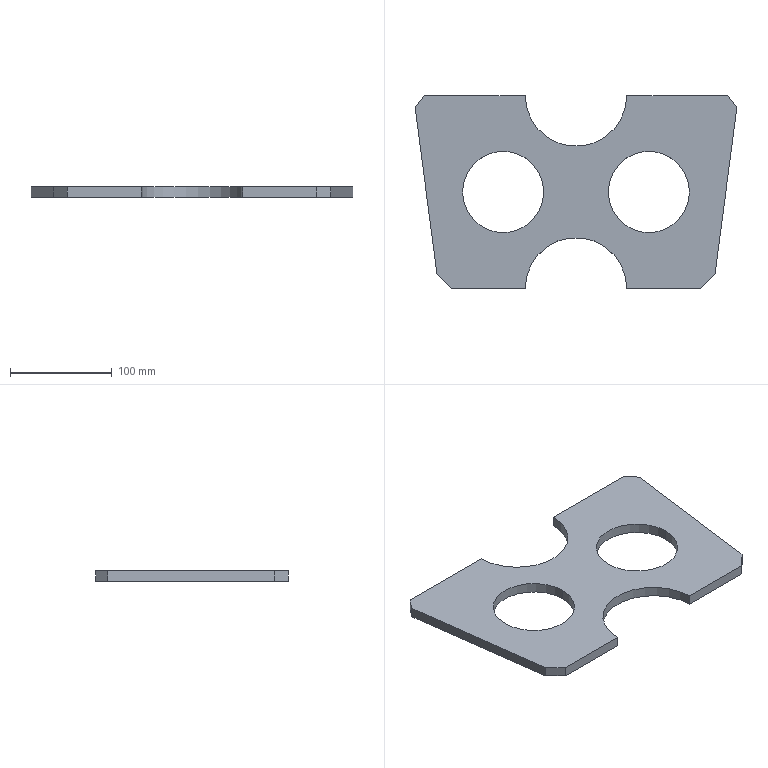Part | SolidWorks | features Extrusion 1 | 1 solid | 18 faces | box 316.869 x 190 x 10 mm | volume 378498 mm3 | plane 12 | cylinder 6 | commonest cylinder face diameters 80 x4 100 x2
STEP:
#1=CARTESIAN_POINT('',(-31.75,0.,10.));
#2=VERTEX_POINT('',#1);
#3=CARTESIAN_POINT('',(-111.75,0.,10.));
#4=VERTEX_POINT('',#3);
#5=CARTESIAN_POINT('',(-71.75,0.,10.));
#6=DIRECTION('',(0.,0.,-1.));
#7=DIRECTION('',(1.,0.,0.));
#8=AXIS2_PLACEMENT_3D('',#5,#6,#7);
#9=CIRCLE('',#8,40.);
#10=EDGE_CURVE('',#2,#4,#9,.T.);
#11=ORIENTED_EDGE('',*,*,#10,.F.);
#12=CARTESIAN_POINT('',(-31.75,0.,0.));
#13=VERTEX_POINT('',#12);
#14=CARTESIAN_POINT('',(-31.75,0.,10.));
#15=DIRECTION('',(0.,0.,-1.));
#16=VECTOR('',#15,1000.);
#17=LINE('',#14,#16);
#18=EDGE_CURVE('',#2,#13,#17,.T.);
#19=ORIENTED_EDGE('',*,*,#18,.T.);
#20=CARTESIAN_POINT('',(-111.75,0.,0.));
#21=VERTEX_POINT('',#20);
#22=CARTESIAN_POINT('',(-71.75,0.,0.));
#23=DIRECTION('',(0.,0.,-1.));
#24=DIRECTION('',(1.,0.,0.));
#25=AXIS2_PLACEMENT_3D('',#22,#23,#24);
#26=CIRCLE('',#25,40.);
#27=EDGE_CURVE('',#13,#21,#26,.T.);
#28=ORIENTED_EDGE('',*,*,#27,.T.);
#29=CARTESIAN_POINT('',(-111.75,0.,10.));
#30=DIRECTION('',(0.,0.,-1.));
#31=VECTOR('',#30,1000.);
#32=LINE('',#29,#31);
#33=EDGE_CURVE('',#4,#21,#32,.T.);
#34=ORIENTED_EDGE('',*,*,#33,.F.);
#35=EDGE_LOOP('',(#11,#19,#28,#34));
#36=FACE_OUTER_BOUND('',#35,.T.);
#37=CARTESIAN_POINT('',(-71.75,0.,10.));
#38=DIRECTION('',(0.,0.,-1.));
#39=DIRECTION('',(-1.,0.,0.));
#40=AXIS2_PLACEMENT_3D('',#37,#38,#39);
#41=CYLINDRICAL_SURFACE('',#40,40.);
#42=ADVANCED_FACE('',(#36),#41,.F.);
#43=CARTESIAN_POINT('',(31.75,0.,10.));
#44=VERTEX_POINT('',#43);
#45=CARTESIAN_POINT('',(111.75,0.,10.));
#46=VERTEX_POINT('',#45);
#47=CARTESIAN_POINT('',(71.75,0.,10.));
#48=DIRECTION('',(0.,0.,1.));
#49=DIRECTION('',(1.,0.,0.));
#50=AXIS2_PLACEMENT_3D('',#47,#48,#49);
#51=CIRCLE('',#50,40.);
#52=EDGE_CURVE('',#44,#46,#51,.T.);
#53=ORIENTED_EDGE('',*,*,#52,.T.);
#54=CARTESIAN_POINT('',(111.75,0.,0.));
#55=VERTEX_POINT('',#54);
#56=CARTESIAN_POINT('',(111.75,0.,10.));
#57=DIRECTION('',(0.,0.,-1.));
#58=VECTOR('',#57,1000.);
#59=LINE('',#56,#58);
#60=EDGE_CURVE('',#46,#55,#59,.T.);
#61=ORIENTED_EDGE('',*,*,#60,.T.);
#62=CARTESIAN_POINT('',(31.75,0.,0.));
#63=VERTEX_POINT('',#62);
#64=CARTESIAN_POINT('',(71.75,0.,0.));
#65=DIRECTION('',(0.,0.,1.));
#66=DIRECTION('',(1.,0.,0.));
#67=AXIS2_PLACEMENT_3D('',#64,#65,#66);
#68=CIRCLE('',#67,40.);
#69=EDGE_CURVE('',#63,#55,#68,.T.);
#70=ORIENTED_EDGE('',*,*,#69,.F.);
#71=CARTESIAN_POINT('',(31.75,0.,10.));
#72=DIRECTION('',(0.,0.,-1.));
#73=VECTOR('',#72,1000.);
#74=LINE('',#71,#73);
#75=EDGE_CURVE('',#44,#63,#74,.T.);
#76=ORIENTED_EDGE('',*,*,#75,.F.);
#77=EDGE_LOOP('',(#53,#61,#70,#76));
#78=FACE_OUTER_BOUND('',#77,.T.);
#79=CARTESIAN_POINT('',(71.75,0.,10.));
#80=DIRECTION('',(0.,0.,-1.));
#81=DIRECTION('',(-1.,0.,0.));
#82=AXIS2_PLACEMENT_3D('',#79,#80,#81);
#83=CYLINDRICAL_SURFACE('',#82,40.);
#84=ADVANCED_FACE('',(#78),#83,.F.);
#85=CARTESIAN_POINT('',(50.,-95.,0.));
#86=VERTEX_POINT('',#85);
#87=CARTESIAN_POINT('',(-50.,-95.,0.));
#88=VERTEX_POINT('',#87);
#89=CARTESIAN_POINT('',(0.,-95.,0.));
#90=DIRECTION('',(0.,0.,1.));
#91=DIRECTION('',(1.,0.,0.));
#92=AXIS2_PLACEMENT_3D('',#89,#90,#91);
#93=CIRCLE('',#92,50.);
#94=EDGE_CURVE('',#86,#88,#93,.T.);
#95=ORIENTED_EDGE('',*,*,#94,.F.);
#96=CARTESIAN_POINT('',(50.,-95.,10.));
#97=VERTEX_POINT('',#96);
#98=CARTESIAN_POINT('',(50.,-95.,10.));
#99=DIRECTION('',(0.,0.,-1.));
#100=VECTOR('',#99,1000.);
#101=LINE('',#98,#100);
#102=EDGE_CURVE('',#97,#86,#101,.T.);
#103=ORIENTED_EDGE('',*,*,#102,.F.);
#104=CARTESIAN_POINT('',(-50.,-95.,10.));
#105=VERTEX_POINT('',#104);
#106=CARTESIAN_POINT('',(0.,-95.,10.));
#107=DIRECTION('',(0.,0.,1.));
#108=DIRECTION('',(1.,0.,0.));
#109=AXIS2_PLACEMENT_3D('',#106,#107,#108);
#110=CIRCLE('',#109,50.);
#111=EDGE_CURVE('',#97,#105,#110,.T.);
#112=ORIENTED_EDGE('',*,*,#111,.T.);
#113=CARTESIAN_POINT('',(-50.,-95.,10.));
#114=DIRECTION('',(0.,0.,-1.));
#115=VECTOR('',#114,1000.);
#116=LINE('',#113,#115);
#117=EDGE_CURVE('',#105,#88,#116,.T.);
#118=ORIENTED_EDGE('',*,*,#117,.T.);
#119=EDGE_LOOP('',(#95,#103,#112,#118));
#120=FACE_OUTER_BOUND('',#119,.T.);
#121=CARTESIAN_POINT('',(0.,-95.,10.));
#122=DIRECTION('',(0.,0.,-1.));
#123=DIRECTION('',(-1.,0.,0.));
#124=AXIS2_PLACEMENT_3D('',#121,#122,#123);
#125=CYLINDRICAL_SURFACE('',#124,50.);
#126=ADVANCED_FACE('',(#120),#125,.F.);
#127=CARTESIAN_POINT('',(123.,-95.,0.));
#128=VERTEX_POINT('',#127);
#129=CARTESIAN_POINT('',(0.,-95.,0.));
#130=DIRECTION('',(1.,0.,0.));
#131=VECTOR('',#130,1000.);
#132=LINE('',#129,#131);
#133=EDGE_CURVE('',#86,#128,#132,.T.);
#134=ORIENTED_EDGE('',*,*,#133,.T.);
#135=CARTESIAN_POINT('',(123.,-95.,10.));
#136=VERTEX_POINT('',#135);
#137=CARTESIAN_POINT('',(123.,-95.,10.));
#138=DIRECTION('',(0.,0.,-1.));
#139=VECTOR('',#138,1000.);
#140=LINE('',#137,#139);
#141=EDGE_CURVE('',#136,#128,#140,.T.);
#142=ORIENTED_EDGE('',*,*,#141,.F.);
#143=CARTESIAN_POINT('',(0.,-95.,10.));
#144=DIRECTION('',(1.,0.,0.));
#145=VECTOR('',#144,1000.);
#146=LINE('',#143,#145);
#147=EDGE_CURVE('',#97,#136,#146,.T.);
#148=ORIENTED_EDGE('',*,*,#147,.F.);
#149=ORIENTED_EDGE('',*,*,#102,.T.);
#150=EDGE_LOOP('',(#134,#142,#148,#149));
#151=FACE_OUTER_BOUND('',#150,.T.);
#152=CARTESIAN_POINT('',(0.,-95.,10.));
#153=DIRECTION('',(0.,1.,0.));
#154=DIRECTION('',(0.,0.,1.));
#155=AXIS2_PLACEMENT_3D('',#152,#153,#154);
#156=PLANE('',#155);
#157=ADVANCED_FACE('',(#151),#156,.F.);
#158=CARTESIAN_POINT('',(136.818,-81.182,0.));
#159=VERTEX_POINT('',#158);
#160=CARTESIAN_POINT('',(-34.76,-252.76,0.));
#161=DIRECTION('',(0.7071,0.7071,0.));
#162=VECTOR('',#161,1000.);
#163=LINE('',#160,#162);
#164=EDGE_CURVE('',#128,#159,#163,.T.);
#165=ORIENTED_EDGE('',*,*,#164,.T.);
#166=CARTESIAN_POINT('',(136.818,-81.182,10.));
#167=VERTEX_POINT('',#166);
#168=CARTESIAN_POINT('',(136.818,-81.182,10.));
#169=DIRECTION('',(0.,0.,-1.));
#170=VECTOR('',#169,1000.);
#171=LINE('',#168,#170);
#172=EDGE_CURVE('',#167,#159,#171,.T.);
#173=ORIENTED_EDGE('',*,*,#172,.F.);
#174=CARTESIAN_POINT('',(-34.76,-252.76,10.));
#175=DIRECTION('',(0.7071,0.7071,0.));
#176=VECTOR('',#175,1000.);
#177=LINE('',#174,#176);
#178=EDGE_CURVE('',#136,#167,#177,.T.);
#179=ORIENTED_EDGE('',*,*,#178,.F.);
#180=ORIENTED_EDGE('',*,*,#141,.T.);
#181=EDGE_LOOP('',(#165,#173,#179,#180));
#182=FACE_OUTER_BOUND('',#181,.T.);
#183=CARTESIAN_POINT('',(-34.76,-252.76,10.));
#184=DIRECTION('',(-0.7071,0.7071,0.));
#185=DIRECTION('',(-0.7071,-0.7071,0.));
#186=AXIS2_PLACEMENT_3D('',#183,#184,#185);
#187=PLANE('',#186);
#188=ADVANCED_FACE('',(#182),#187,.F.);
#189=CARTESIAN_POINT('',(158.435,83.103,0.));
#190=VERTEX_POINT('',#189);
#191=CARTESIAN_POINT('',(107.802,-301.704,0.));
#192=DIRECTION('',(-0.1305,-0.9915,0.));
#193=VECTOR('',#192,1000.);
#194=LINE('',#191,#193);
#195=EDGE_CURVE('',#190,#159,#194,.T.);
#196=ORIENTED_EDGE('',*,*,#195,.F.);
#197=CARTESIAN_POINT('',(158.435,83.103,10.));
#198=VERTEX_POINT('',#197);
#199=CARTESIAN_POINT('',(158.435,83.103,10.));
#200=DIRECTION('',(0.,0.,-1.));
#201=VECTOR('',#200,1000.);
#202=LINE('',#199,#201);
#203=EDGE_CURVE('',#198,#190,#202,.T.);
#204=ORIENTED_EDGE('',*,*,#203,.F.);
#205=CARTESIAN_POINT('',(107.802,-301.704,10.));
#206=DIRECTION('',(-0.1305,-0.9915,0.));
#207=VECTOR('',#206,1000.);
#208=LINE('',#205,#207);
#209=EDGE_CURVE('',#198,#167,#208,.T.);
#210=ORIENTED_EDGE('',*,*,#209,.T.);
#211=ORIENTED_EDGE('',*,*,#172,.T.);
#212=EDGE_LOOP('',(#196,#204,#210,#211));
#213=FACE_OUTER_BOUND('',#212,.T.);
#214=CARTESIAN_POINT('',(107.802,-301.704,10.));
#215=DIRECTION('',(0.9915,-0.1305,0.));
#216=DIRECTION('',(0.1305,0.9915,0.));
#217=AXIS2_PLACEMENT_3D('',#214,#215,#216);
#218=PLANE('',#217);
#219=ADVANCED_FACE('',(#213),#218,.T.);
#220=CARTESIAN_POINT('',(149.304,95.,0.));
#221=VERTEX_POINT('',#220);
#222=CARTESIAN_POINT('',(278.713,-73.624,0.));
#223=DIRECTION('',(0.6088,-0.7933,0.));
#224=VECTOR('',#223,1000.);
#225=LINE('',#222,#224);
#226=EDGE_CURVE('',#221,#190,#225,.T.);
#227=ORIENTED_EDGE('',*,*,#226,.F.);
#228=CARTESIAN_POINT('',(149.304,95.,10.));
#229=VERTEX_POINT('',#228);
#230=CARTESIAN_POINT('',(149.304,95.,10.));
#231=DIRECTION('',(0.,0.,-1.));
#232=VECTOR('',#231,1000.);
#233=LINE('',#230,#232);
#234=EDGE_CURVE('',#229,#221,#233,.T.);
#235=ORIENTED_EDGE('',*,*,#234,.F.);
#236=CARTESIAN_POINT('',(278.713,-73.624,10.));
#237=DIRECTION('',(0.6088,-0.7933,0.));
#238=VECTOR('',#237,1000.);
#239=LINE('',#236,#238);
#240=EDGE_CURVE('',#229,#198,#239,.T.);
#241=ORIENTED_EDGE('',*,*,#240,.T.);
#242=ORIENTED_EDGE('',*,*,#203,.T.);
#243=EDGE_LOOP('',(#227,#235,#241,#242));
#244=FACE_OUTER_BOUND('',#243,.T.);
#245=CARTESIAN_POINT('',(278.713,-73.624,10.));
#246=DIRECTION('',(0.7933,0.6088,0.));
#247=DIRECTION('',(-0.6088,0.7933,0.));
#248=AXIS2_PLACEMENT_3D('',#245,#246,#247);
#249=PLANE('',#248);
#250=ADVANCED_FACE('',(#244),#249,.T.);
#251=CARTESIAN_POINT('',(50.,95.,0.));
#252=VERTEX_POINT('',#251);
#253=CARTESIAN_POINT('',(0.,95.,0.));
#254=DIRECTION('',(1.,0.,0.));
#255=VECTOR('',#254,1000.);
#256=LINE('',#253,#255);
#257=EDGE_CURVE('',#252,#221,#256,.T.);
#258=ORIENTED_EDGE('',*,*,#257,.F.);
#259=CARTESIAN_POINT('',(50.,95.,10.));
#260=VERTEX_POINT('',#259);
#261=CARTESIAN_POINT('',(50.,95.,10.));
#262=DIRECTION('',(0.,0.,-1.));
#263=VECTOR('',#262,1000.);
#264=LINE('',#261,#263);
#265=EDGE_CURVE('',#260,#252,#264,.T.);
#266=ORIENTED_EDGE('',*,*,#265,.F.);
#267=CARTESIAN_POINT('',(0.,95.,10.));
#268=DIRECTION('',(1.,0.,0.));
#269=VECTOR('',#268,1000.);
#270=LINE('',#267,#269);
#271=EDGE_CURVE('',#260,#229,#270,.T.);
#272=ORIENTED_EDGE('',*,*,#271,.T.);
#273=ORIENTED_EDGE('',*,*,#234,.T.);
#274=EDGE_LOOP('',(#258,#266,#272,#273));
#275=FACE_OUTER_BOUND('',#274,.T.);
#276=CARTESIAN_POINT('',(0.,95.,10.));
#277=DIRECTION('',(0.,1.,0.));
#278=DIRECTION('',(0.,0.,1.));
#279=AXIS2_PLACEMENT_3D('',#276,#277,#278);
#280=PLANE('',#279);
#281=ADVANCED_FACE('',(#275),#280,.T.);
#282=CARTESIAN_POINT('',(-50.,95.,0.));
#283=VERTEX_POINT('',#282);
#284=CARTESIAN_POINT('',(0.,95.,0.));
#285=DIRECTION('',(0.,0.,1.));
#286=DIRECTION('',(1.,0.,0.));
#287=AXIS2_PLACEMENT_3D('',#284,#285,#286);
#288=CIRCLE('',#287,50.);
#289=EDGE_CURVE('',#283,#252,#288,.T.);
#290=ORIENTED_EDGE('',*,*,#289,.F.);
#291=CARTESIAN_POINT('',(-50.,95.,10.));
#292=VERTEX_POINT('',#291);
#293=CARTESIAN_POINT('',(-50.,95.,10.));
#294=DIRECTION('',(0.,0.,-1.));
#295=VECTOR('',#294,1000.);
#296=LINE('',#293,#295);
#297=EDGE_CURVE('',#292,#283,#296,.T.);
#298=ORIENTED_EDGE('',*,*,#297,.F.);
#299=CARTESIAN_POINT('',(0.,95.,10.));
#300=DIRECTION('',(0.,0.,1.));
#301=DIRECTION('',(1.,0.,0.));
#302=AXIS2_PLACEMENT_3D('',#299,#300,#301);
#303=CIRCLE('',#302,50.);
#304=EDGE_CURVE('',#292,#260,#303,.T.);
#305=ORIENTED_EDGE('',*,*,#304,.T.);
#306=ORIENTED_EDGE('',*,*,#265,.T.);
#307=EDGE_LOOP('',(#290,#298,#305,#306));
#308=FACE_OUTER_BOUND('',#307,.T.);
#309=CARTESIAN_POINT('',(0.,95.,10.));
#310=DIRECTION('',(0.,0.,-1.));
#311=DIRECTION('',(-1.,0.,0.));
#312=AXIS2_PLACEMENT_3D('',#309,#310,#311);
#313=CYLINDRICAL_SURFACE('',#312,50.);
#314=ADVANCED_FACE('',(#308),#313,.F.);
#315=CARTESIAN_POINT('',(-149.304,95.,0.));
#316=VERTEX_POINT('',#315);
#317=CARTESIAN_POINT('',(0.,95.,0.));
#318=DIRECTION('',(-1.,0.,0.));
#319=VECTOR('',#318,1000.);
#320=LINE('',#317,#319);
#321=EDGE_CURVE('',#283,#316,#320,.T.);
#322=ORIENTED_EDGE('',*,*,#321,.T.);
#323=CARTESIAN_POINT('',(-149.304,95.,10.));
#324=VERTEX_POINT('',#323);
#325=CARTESIAN_POINT('',(-149.304,95.,10.));
#326=DIRECTION('',(0.,0.,-1.));
#327=VECTOR('',#326,1000.);
#328=LINE('',#325,#327);
#329=EDGE_CURVE('',#324,#316,#328,.T.);
#330=ORIENTED_EDGE('',*,*,#329,.F.);
#331=CARTESIAN_POINT('',(0.,95.,10.));
#332=DIRECTION('',(-1.,0.,0.));
#333=VECTOR('',#332,1000.);
#334=LINE('',#331,#333);
#335=EDGE_CURVE('',#292,#324,#334,.T.);
#336=ORIENTED_EDGE('',*,*,#335,.F.);
#337=ORIENTED_EDGE('',*,*,#297,.T.);
#338=EDGE_LOOP('',(#322,#330,#336,#337));
#339=FACE_OUTER_BOUND('',#338,.T.);
#340=CARTESIAN_POINT('',(0.,95.,10.));
#341=DIRECTION('',(0.,-1.,0.));
#342=DIRECTION('',(0.,0.,-1.));
#343=AXIS2_PLACEMENT_3D('',#340,#341,#342);
#344=PLANE('',#343);
#345=ADVANCED_FACE('',(#339),#344,.F.);
#346=CARTESIAN_POINT('',(-158.435,83.103,0.));
#347=VERTEX_POINT('',#346);
#348=CARTESIAN_POINT('',(-278.713,-73.624,0.));
#349=DIRECTION('',(-0.6088,-0.7933,0.));
#350=VECTOR('',#349,1000.);
#351=LINE('',#348,#350);
#352=EDGE_CURVE('',#316,#347,#351,.T.);
#353=ORIENTED_EDGE('',*,*,#352,.T.);
#354=CARTESIAN_POINT('',(-158.435,83.103,10.));
#355=VERTEX_POINT('',#354);
#356=CARTESIAN_POINT('',(-158.435,83.103,10.));
#357=DIRECTION('',(0.,0.,-1.));
#358=VECTOR('',#357,1000.);
#359=LINE('',#356,#358);
#360=EDGE_CURVE('',#355,#347,#359,.T.);
#361=ORIENTED_EDGE('',*,*,#360,.F.);
#362=CARTESIAN_POINT('',(-278.713,-73.624,10.));
#363=DIRECTION('',(-0.6088,-0.7933,0.));
#364=VECTOR('',#363,1000.);
#365=LINE('',#362,#364);
#366=EDGE_CURVE('',#324,#355,#365,.T.);
#367=ORIENTED_EDGE('',*,*,#366,.F.);
#368=ORIENTED_EDGE('',*,*,#329,.T.);
#369=EDGE_LOOP('',(#353,#361,#367,#368));
#370=FACE_OUTER_BOUND('',#369,.T.);
#371=CARTESIAN_POINT('',(-278.713,-73.624,10.));
#372=DIRECTION('',(0.7933,-0.6088,0.));
#373=DIRECTION('',(0.6088,0.7933,0.));
#374=AXIS2_PLACEMENT_3D('',#371,#372,#373);
#375=PLANE('',#374);
#376=ADVANCED_FACE('',(#370),#375,.F.);
#377=CARTESIAN_POINT('',(-136.818,-81.182,0.));
#378=VERTEX_POINT('',#377);
#379=CARTESIAN_POINT('',(-107.802,-301.704,0.));
#380=DIRECTION('',(0.1305,-0.9915,0.));
#381=VECTOR('',#380,1000.);
#382=LINE('',#379,#381);
#383=EDGE_CURVE('',#347,#378,#382,.T.);
#384=ORIENTED_EDGE('',*,*,#383,.T.);
#385=CARTESIAN_POINT('',(-136.818,-81.182,10.));
#386=VERTEX_POINT('',#385);
#387=CARTESIAN_POINT('',(-136.818,-81.182,10.));
#388=DIRECTION('',(0.,0.,-1.));
#389=VECTOR('',#388,1000.);
#390=LINE('',#387,#389);
#391=EDGE_CURVE('',#386,#378,#390,.T.);
#392=ORIENTED_EDGE('',*,*,#391,.F.);
#393=CARTESIAN_POINT('',(-107.802,-301.704,10.));
#394=DIRECTION('',(0.1305,-0.9915,0.));
#395=VECTOR('',#394,1000.);
#396=LINE('',#393,#395);
#397=EDGE_CURVE('',#355,#386,#396,.T.);
#398=ORIENTED_EDGE('',*,*,#397,.F.);
#399=ORIENTED_EDGE('',*,*,#360,.T.);
#400=EDGE_LOOP('',(#384,#392,#398,#399));
#401=FACE_OUTER_BOUND('',#400,.T.);
#402=CARTESIAN_POINT('',(-107.802,-301.704,10.));
#403=DIRECTION('',(0.9915,0.1305,0.));
#404=DIRECTION('',(-0.1305,0.9915,0.));
#405=AXIS2_PLACEMENT_3D('',#402,#403,#404);
#406=PLANE('',#405);
#407=ADVANCED_FACE('',(#401),#406,.F.);
#408=CARTESIAN_POINT('',(-123.,-95.,0.));
#409=VERTEX_POINT('',#408);
#410=CARTESIAN_POINT('',(34.76,-252.76,0.));
#411=DIRECTION('',(-0.7071,0.7071,0.));
#412=VECTOR('',#411,1000.);
#413=LINE('',#410,#412);
#414=EDGE_CURVE('',#409,#378,#413,.T.);
#415=ORIENTED_EDGE('',*,*,#414,.F.);
#416=CARTESIAN_POINT('',(-123.,-95.,10.));
#417=VERTEX_POINT('',#416);
#418=CARTESIAN_POINT('',(-123.,-95.,10.));
#419=DIRECTION('',(0.,0.,-1.));
#420=VECTOR('',#419,1000.);
#421=LINE('',#418,#420);
#422=EDGE_CURVE('',#417,#409,#421,.T.);
#423=ORIENTED_EDGE('',*,*,#422,.F.);
#424=CARTESIAN_POINT('',(34.76,-252.76,10.));
#425=DIRECTION('',(-0.7071,0.7071,0.));
#426=VECTOR('',#425,1000.);
#427=LINE('',#424,#426);
#428=EDGE_CURVE('',#417,#386,#427,.T.);
#429=ORIENTED_EDGE('',*,*,#428,.T.);
#430=ORIENTED_EDGE('',*,*,#391,.T.);
#431=EDGE_LOOP('',(#415,#423,#429,#430));
#432=FACE_OUTER_BOUND('',#431,.T.);
#433=CARTESIAN_POINT('',(34.76,-252.76,10.));
#434=DIRECTION('',(-0.7071,-0.7071,0.));
#435=DIRECTION('',(0.7071,-0.7071,0.));
#436=AXIS2_PLACEMENT_3D('',#433,#434,#435);
#437=PLANE('',#436);
#438=ADVANCED_FACE('',(#432),#437,.T.);
#439=CARTESIAN_POINT('',(0.,-95.,0.));
#440=DIRECTION('',(-1.,0.,0.));
#441=VECTOR('',#440,1000.);
#442=LINE('',#439,#441);
#443=EDGE_CURVE('',#88,#409,#442,.T.);
#444=ORIENTED_EDGE('',*,*,#443,.F.);
#445=ORIENTED_EDGE('',*,*,#117,.F.);
#446=CARTESIAN_POINT('',(0.,-95.,10.));
#447=DIRECTION('',(-1.,0.,0.));
#448=VECTOR('',#447,1000.);
#449=LINE('',#446,#448);
#450=EDGE_CURVE('',#105,#417,#449,.T.);
#451=ORIENTED_EDGE('',*,*,#450,.T.);
#452=ORIENTED_EDGE('',*,*,#422,.T.);
#453=EDGE_LOOP('',(#444,#445,#451,#452));
#454=FACE_OUTER_BOUND('',#453,.T.);
#455=CARTESIAN_POINT('',(0.,-95.,10.));
#456=DIRECTION('',(0.,-1.,0.));
#457=DIRECTION('',(0.,0.,-1.));
#458=AXIS2_PLACEMENT_3D('',#455,#456,#457);
#459=PLANE('',#458);
#460=ADVANCED_FACE('',(#454),#459,.T.);
#461=ORIENTED_EDGE('',*,*,#60,.F.);
#462=CARTESIAN_POINT('',(71.75,0.,10.));
#463=DIRECTION('',(0.,0.,1.));
#464=DIRECTION('',(1.,0.,0.));
#465=AXIS2_PLACEMENT_3D('',#462,#463,#464);
#466=CIRCLE('',#465,40.);
#467=EDGE_CURVE('',#46,#44,#466,.T.);
#468=ORIENTED_EDGE('',*,*,#467,.T.);
#469=ORIENTED_EDGE('',*,*,#75,.T.);
#470=CARTESIAN_POINT('',(71.75,0.,0.));
#471=DIRECTION('',(0.,0.,1.));
#472=DIRECTION('',(1.,0.,0.));
#473=AXIS2_PLACEMENT_3D('',#470,#471,#472);
#474=CIRCLE('',#473,40.);
#475=EDGE_CURVE('',#55,#63,#474,.T.);
#476=ORIENTED_EDGE('',*,*,#475,.F.);
#477=EDGE_LOOP('',(#461,#468,#469,#476));
#478=FACE_OUTER_BOUND('',#477,.T.);
#479=CARTESIAN_POINT('',(71.75,0.,10.));
#480=DIRECTION('',(0.,0.,-1.));
#481=DIRECTION('',(-1.,0.,0.));
#482=AXIS2_PLACEMENT_3D('',#479,#480,#481);
#483=CYLINDRICAL_SURFACE('',#482,40.);
#484=ADVANCED_FACE('',(#478),#483,.F.);
#485=ORIENTED_EDGE('',*,*,#18,.F.);
#486=CARTESIAN_POINT('',(-71.75,0.,10.));
#487=DIRECTION('',(0.,0.,-1.));
#488=DIRECTION('',(1.,0.,0.));
#489=AXIS2_PLACEMENT_3D('',#486,#487,#488);
#490=CIRCLE('',#489,40.);
#491=EDGE_CURVE('',#4,#2,#490,.T.);
#492=ORIENTED_EDGE('',*,*,#491,.F.);
#493=ORIENTED_EDGE('',*,*,#33,.T.);
#494=CARTESIAN_POINT('',(-71.75,0.,0.));
#495=DIRECTION('',(0.,0.,-1.));
#496=DIRECTION('',(1.,0.,0.));
#497=AXIS2_PLACEMENT_3D('',#494,#495,#496);
#498=CIRCLE('',#497,40.);
#499=EDGE_CURVE('',#21,#13,#498,.T.);
#500=ORIENTED_EDGE('',*,*,#499,.T.);
#501=EDGE_LOOP('',(#485,#492,#493,#500));
#502=FACE_OUTER_BOUND('',#501,.T.);
#503=CARTESIAN_POINT('',(-71.75,0.,10.));
#504=DIRECTION('',(0.,0.,-1.));
#505=DIRECTION('',(-1.,0.,0.));
#506=AXIS2_PLACEMENT_3D('',#503,#504,#505);
#507=CYLINDRICAL_SURFACE('',#506,40.);
#508=ADVANCED_FACE('',(#502),#507,.F.);
#509=ORIENTED_EDGE('',*,*,#52,.F.);
#510=ORIENTED_EDGE('',*,*,#467,.F.);
#511=EDGE_LOOP('',(#509,#510));
#512=FACE_BOUND('',#511,.T.);
#513=ORIENTED_EDGE('',*,*,#111,.F.);
#514=ORIENTED_EDGE('',*,*,#147,.T.);
#515=ORIENTED_EDGE('',*,*,#178,.T.);
#516=ORIENTED_EDGE('',*,*,#209,.F.);
#517=ORIENTED_EDGE('',*,*,#240,.F.);
#518=ORIENTED_EDGE('',*,*,#271,.F.);
#519=ORIENTED_EDGE('',*,*,#304,.F.);
#520=ORIENTED_EDGE('',*,*,#335,.T.);
#521=ORIENTED_EDGE('',*,*,#366,.T.);
#522=ORIENTED_EDGE('',*,*,#397,.T.);
#523=ORIENTED_EDGE('',*,*,#428,.F.);
#524=ORIENTED_EDGE('',*,*,#450,.F.);
#525=EDGE_LOOP('',(#513,#514,#515,#516,#517,#518,#519,#520,#521,#522,#523,#524));
#526=FACE_OUTER_BOUND('',#525,.T.);
#527=ORIENTED_EDGE('',*,*,#491,.T.);
#528=ORIENTED_EDGE('',*,*,#10,.T.);
#529=EDGE_LOOP('',(#527,#528));
#530=FACE_BOUND('',#529,.T.);
#531=CARTESIAN_POINT('',(0.,-287.519,10.));
#532=DIRECTION('',(0.,0.,1.));
#533=DIRECTION('',(1.,0.,0.));
#534=AXIS2_PLACEMENT_3D('',#531,#532,#533);
#535=PLANE('',#534);
#536=ADVANCED_FACE('',(#512,#526,#530),#535,.T.);
#537=ORIENTED_EDGE('',*,*,#69,.T.);
#538=ORIENTED_EDGE('',*,*,#475,.T.);
#539=EDGE_LOOP('',(#537,#538));
#540=FACE_BOUND('',#539,.T.);
#541=ORIENTED_EDGE('',*,*,#94,.T.);
#542=ORIENTED_EDGE('',*,*,#443,.T.);
#543=ORIENTED_EDGE('',*,*,#414,.T.);
#544=ORIENTED_EDGE('',*,*,#383,.F.);
#545=ORIENTED_EDGE('',*,*,#352,.F.);
#546=ORIENTED_EDGE('',*,*,#321,.F.);
#547=ORIENTED_EDGE('',*,*,#289,.T.);
#548=ORIENTED_EDGE('',*,*,#257,.T.);
#549=ORIENTED_EDGE('',*,*,#226,.T.);
#550=ORIENTED_EDGE('',*,*,#195,.T.);
#551=ORIENTED_EDGE('',*,*,#164,.F.);
#552=ORIENTED_EDGE('',*,*,#133,.F.);
#553=EDGE_LOOP('',(#541,#542,#543,#544,#545,#546,#547,#548,#549,#550,#551,#552));
#554=FACE_OUTER_BOUND('',#553,.T.);
#555=ORIENTED_EDGE('',*,*,#499,.F.);
#556=ORIENTED_EDGE('',*,*,#27,.F.);
#557=EDGE_LOOP('',(#555,#556));
#558=FACE_BOUND('',#557,.T.);
#559=CARTESIAN_POINT('',(0.,-287.519,0.));
#560=DIRECTION('',(0.,0.,1.));
#561=DIRECTION('',(1.,0.,0.));
#562=AXIS2_PLACEMENT_3D('',#559,#560,#561);
#563=PLANE('',#562);
#564=ADVANCED_FACE('',(#540,#554,#558),#563,.F.);
#565=CLOSED_SHELL('',(#42,#84,#126,#157,#188,#219,#250,#281,#314,#345,#376,#407,#438,#460,#484,#508,#536,#564));
#566=MANIFOLD_SOLID_BREP('',#565);
#567=CARTESIAN_POINT('',(0.,0.,0.));
#568=DIRECTION('',(0.,0.,1.));
#569=DIRECTION('',(1.,0.,0.));
#570=AXIS2_PLACEMENT_3D('',#567,#568,#569);
#571=(LENGTH_UNIT()NAMED_UNIT(*)SI_UNIT(.MILLI.,.METRE.));
#572=UNCERTAINTY_MEASURE_WITH_UNIT(LENGTH_MEASURE(0.00001),#571,'','');
#573=(NAMED_UNIT(*)PLANE_ANGLE_UNIT()SI_UNIT($,.RADIAN.));
#574=(NAMED_UNIT(*)SI_UNIT($,.STERADIAN.)SOLID_ANGLE_UNIT());
#575=(GEOMETRIC_REPRESENTATION_CONTEXT(3)GLOBAL_UNCERTAINTY_ASSIGNED_CONTEXT((#572))GLOBAL_UNIT_ASSIGNED_CONTEXT((#571,#573,#574))REPRESENTATION_CONTEXT('',''));
#576=ADVANCED_BREP_SHAPE_REPRESENTATION('',(#566,#570),#575);